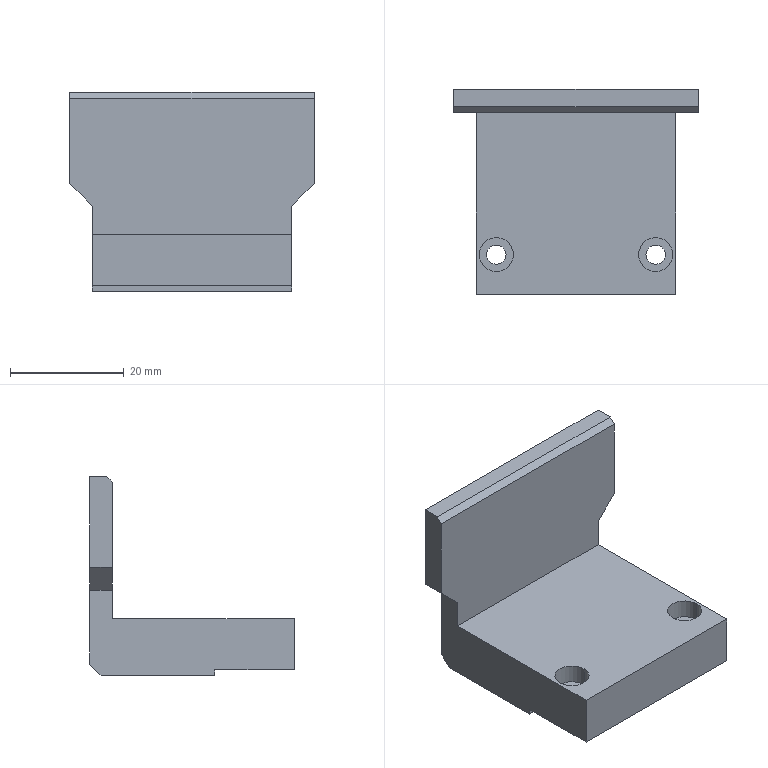Part | STEP file | PN_0029 Mount electronic clip connecting plate 1 | 1 solid | 26 faces | box 43 x 36 x 35 mm | volume 15801 mm3 | plane 18 | cylinder 8 | commonest cylinder face diameters 3.4 x4 6 x4